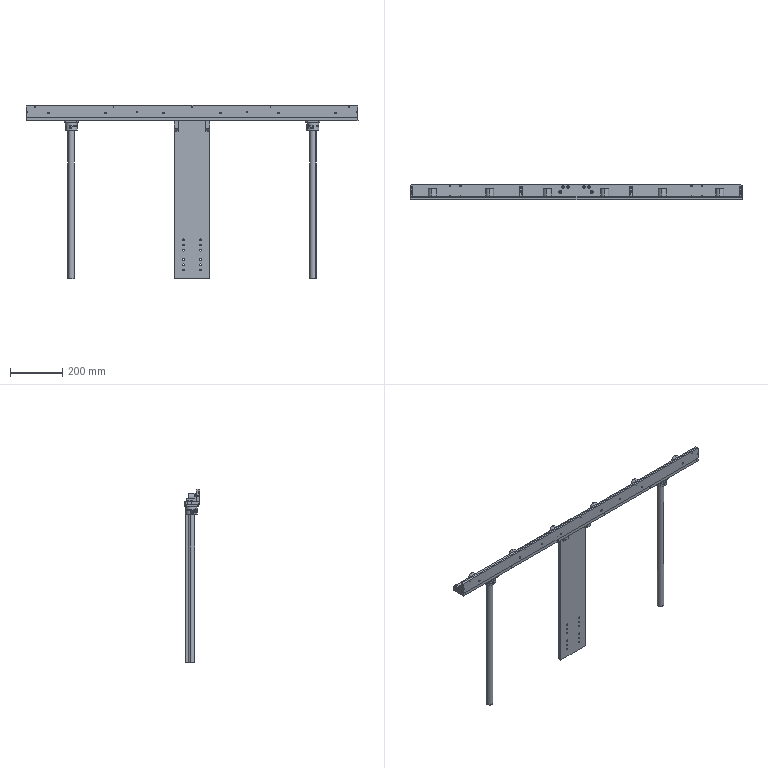Part | SolidWorks | features ReferencePattern 7, DerivedHolePattern 1, MirrorCompFeat 1 | 28 solids | 1029 faces | box 1270 x 60 x 664 mm | volume 3435142 mm3 | cylinder 560 | plane 313 | spline 96 | cone 60 | commonest cylinder face diameters 6.6 x60 8 x52 9 x52 5 x48 18 x48 19 x48